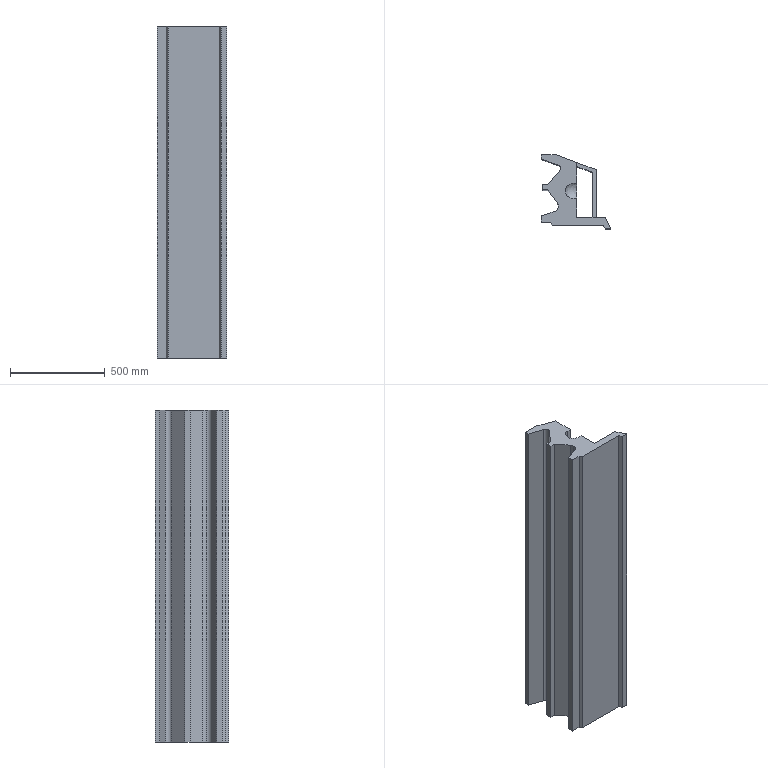Part | SolidWorks | features 3DProfileFeature 2, ICE 2, Extrusion 1, MirrorPattern 1, RevCut 1 | 1 solid | 43 faces | box 368.945 x 388.507 x 1750 mm | volume 104894918 mm3 | plane 34 | cylinder 5 | spline 2 | sphere 2 | commonest cylinder face diameters 80 x3 63.152 x2
STEP:
#1=CARTESIAN_POINT('',(-20.,75.504,-1650.));
#2=VERTEX_POINT('',#1);
#3=CARTESIAN_POINT('',(-60.,35.504,-1650.));
#4=VERTEX_POINT('',#3);
#5=CARTESIAN_POINT('',(-20.,35.504,-1650.));
#6=DIRECTION('',(0.,0.,1.));
#7=DIRECTION('',(-1.,0.,0.));
#8=AXIS2_PLACEMENT_3D('',#5,#6,#7);
#9=CIRCLE('',#8,40.);
#10=EDGE_CURVE('',#2,#4,#9,.T.);
#11=ORIENTED_EDGE('',*,*,#10,.T.);
#12=CARTESIAN_POINT('',(-60.,35.504,-1750.));
#13=VERTEX_POINT('',#12);
#14=CARTESIAN_POINT('',(-60.,35.504,-1650.));
#15=DIRECTION('',(0.,0.,-1.));
#16=VECTOR('',#15,1000.);
#17=LINE('',#14,#16);
#18=EDGE_CURVE('',#4,#13,#17,.T.);
#19=ORIENTED_EDGE('',*,*,#18,.T.);
#20=CARTESIAN_POINT('',(-20.,75.504,-1750.));
#21=VERTEX_POINT('',#20);
#22=CARTESIAN_POINT('',(-20.,35.504,-1750.));
#23=DIRECTION('',(0.,0.,1.));
#24=DIRECTION('',(-1.,0.,0.));
#25=AXIS2_PLACEMENT_3D('',#22,#23,#24);
#26=CIRCLE('',#25,40.);
#27=EDGE_CURVE('',#21,#13,#26,.T.);
#28=ORIENTED_EDGE('',*,*,#27,.F.);
#29=CARTESIAN_POINT('',(-20.,75.504,-1650.));
#30=DIRECTION('',(0.,0.,-1.));
#31=VECTOR('',#30,1000.);
#32=LINE('',#29,#31);
#33=EDGE_CURVE('',#2,#21,#32,.T.);
#34=ORIENTED_EDGE('',*,*,#33,.F.);
#35=EDGE_LOOP('',(#11,#19,#28,#34));
#36=FACE_OUTER_BOUND('',#35,.T.);
#37=CARTESIAN_POINT('',(-20.,35.504,-1650.));
#38=DIRECTION('',(0.,0.,-1.));
#39=DIRECTION('',(-1.,0.,0.));
#40=AXIS2_PLACEMENT_3D('',#37,#38,#39);
#41=CYLINDRICAL_SURFACE('',#40,40.);
#42=ADVANCED_FACE('',(#36),#41,.F.);
#43=CARTESIAN_POINT('',(-95.432,-44.492,-1750.));
#44=VERTEX_POINT('',#43);
#45=CARTESIAN_POINT('',(-102.008,-25.204,-1750.));
#46=VERTEX_POINT('',#45);
#47=CARTESIAN_POINT('',(-127.008,-44.492,-1750.));
#48=DIRECTION('',(0.,0.,1.));
#49=DIRECTION('',(1.,0.,0.));
#50=AXIS2_PLACEMENT_3D('',#47,#48,#49);
#51=CIRCLE('',#50,31.576);
#52=EDGE_CURVE('',#44,#46,#51,.T.);
#53=ORIENTED_EDGE('',*,*,#52,.F.);
#54=CARTESIAN_POINT('',(-95.432,-44.492,0.));
#55=VERTEX_POINT('',#54);
#56=CARTESIAN_POINT('',(-95.432,-44.492,-1750.));
#57=DIRECTION('',(0.,0.,1.));
#58=VECTOR('',#57,1000.);
#59=LINE('',#56,#58);
#60=EDGE_CURVE('',#44,#55,#59,.T.);
#61=ORIENTED_EDGE('',*,*,#60,.T.);
#62=CARTESIAN_POINT('',(-102.008,-25.204,0.));
#63=VERTEX_POINT('',#62);
#64=CARTESIAN_POINT('',(-127.008,-44.492,0.));
#65=DIRECTION('',(0.,0.,1.));
#66=DIRECTION('',(1.,0.,0.));
#67=AXIS2_PLACEMENT_3D('',#64,#65,#66);
#68=CIRCLE('',#67,31.576);
#69=EDGE_CURVE('',#55,#63,#68,.T.);
#70=ORIENTED_EDGE('',*,*,#69,.T.);
#71=CARTESIAN_POINT('',(-102.008,-25.204,-1750.));
#72=DIRECTION('',(0.,0.,1.));
#73=VECTOR('',#72,1000.);
#74=LINE('',#71,#73);
#75=EDGE_CURVE('',#46,#63,#74,.T.);
#76=ORIENTED_EDGE('',*,*,#75,.F.);
#77=EDGE_LOOP('',(#53,#61,#70,#76));
#78=FACE_OUTER_BOUND('',#77,.T.);
#79=CARTESIAN_POINT('',(-127.008,-44.492,-1750.));
#80=DIRECTION('',(0.,0.,1.));
#81=DIRECTION('',(1.,0.,0.));
#82=AXIS2_PLACEMENT_3D('',#79,#80,#81);
#83=CYLINDRICAL_SURFACE('',#82,31.576);
#84=ADVANCED_FACE('',(#78),#83,.F.);
#85=CARTESIAN_POINT('',(0.,185.504,-1590.));
#86=VERTEX_POINT('',#85);
#87=CARTESIAN_POINT('',(0.,164.598,-1590.));
#88=VERTEX_POINT('',#87);
#89=CARTESIAN_POINT('',(0.,164.598,-1590.));
#90=DIRECTION('',(0.,-1.,0.));
#91=VECTOR('',#90,1000.);
#92=LINE('',#89,#91);
#93=EDGE_CURVE('',#86,#88,#92,.T.);
#94=ORIENTED_EDGE('',*,*,#93,.T.);
#95=CARTESIAN_POINT('',(0.,164.598,-160.));
#96=VERTEX_POINT('',#95);
#97=CARTESIAN_POINT('',(0.,164.598,-1590.));
#98=DIRECTION('',(0.,0.,1.));
#99=VECTOR('',#98,1000.);
#100=LINE('',#97,#99);
#101=EDGE_CURVE('',#88,#96,#100,.T.);
#102=ORIENTED_EDGE('',*,*,#101,.T.);
#103=CARTESIAN_POINT('',(0.,185.504,-160.));
#104=VERTEX_POINT('',#103);
#105=CARTESIAN_POINT('',(0.,164.598,-160.));
#106=DIRECTION('',(0.,-1.,0.));
#107=VECTOR('',#106,1000.);
#108=LINE('',#105,#107);
#109=EDGE_CURVE('',#104,#96,#108,.T.);
#110=ORIENTED_EDGE('',*,*,#109,.F.);
#111=CARTESIAN_POINT('',(0.,185.504,0.));
#112=VERTEX_POINT('',#111);
#113=CARTESIAN_POINT('',(0.,185.504,-1750.));
#114=DIRECTION('',(0.,0.,1.));
#115=VECTOR('',#114,1000.);
#116=LINE('',#113,#115);
#117=EDGE_CURVE('',#104,#112,#116,.T.);
#118=ORIENTED_EDGE('',*,*,#117,.T.);
#119=CARTESIAN_POINT('',(0.,75.504,0.));
#120=VERTEX_POINT('',#119);
#121=CARTESIAN_POINT('',(0.,0.,0.));
#122=DIRECTION('',(0.,-1.,0.));
#123=VECTOR('',#122,1000.);
#124=LINE('',#121,#123);
#125=EDGE_CURVE('',#112,#120,#124,.T.);
#126=ORIENTED_EDGE('',*,*,#125,.T.);
#127=CARTESIAN_POINT('',(0.,75.504,-100.));
#128=VERTEX_POINT('',#127);
#129=CARTESIAN_POINT('',(0.,75.504,-100.));
#130=DIRECTION('',(0.,0.,1.));
#131=VECTOR('',#130,1000.);
#132=LINE('',#129,#131);
#133=EDGE_CURVE('',#128,#120,#132,.T.);
#134=ORIENTED_EDGE('',*,*,#133,.F.);
#135=CARTESIAN_POINT('',(0.,95.504,-100.));
#136=VERTEX_POINT('',#135);
#137=CARTESIAN_POINT('',(0.,95.504,-100.));
#138=DIRECTION('',(0.,-1.,0.));
#139=VECTOR('',#138,1000.);
#140=LINE('',#137,#139);
#141=EDGE_CURVE('',#136,#128,#140,.T.);
#142=ORIENTED_EDGE('',*,*,#141,.F.);
#143=CARTESIAN_POINT('',(0.,-24.496,-100.));
#144=VERTEX_POINT('',#143);
#145=CARTESIAN_POINT('',(0.,35.504,-100.));
#146=DIRECTION('',(1.,0.,0.));
#147=DIRECTION('',(0.,-1.,0.));
#148=AXIS2_PLACEMENT_3D('',#145,#146,#147);
#149=CIRCLE('',#148,60.);
#150=EDGE_CURVE('',#144,#136,#149,.T.);
#151=ORIENTED_EDGE('',*,*,#150,.F.);
#152=CARTESIAN_POINT('',(0.,-4.496,-100.));
#153=VERTEX_POINT('',#152);
#154=CARTESIAN_POINT('',(0.,95.504,-100.));
#155=DIRECTION('',(0.,-1.,0.));
#156=VECTOR('',#155,1000.);
#157=LINE('',#154,#156);
#158=EDGE_CURVE('',#153,#144,#157,.T.);
#159=ORIENTED_EDGE('',*,*,#158,.F.);
#160=CARTESIAN_POINT('',(0.,-4.496,0.));
#161=VERTEX_POINT('',#160);
#162=CARTESIAN_POINT('',(0.,-4.496,-100.));
#163=DIRECTION('',(0.,0.,1.));
#164=VECTOR('',#163,1000.);
#165=LINE('',#162,#164);
#166=EDGE_CURVE('',#153,#161,#165,.T.);
#167=ORIENTED_EDGE('',*,*,#166,.T.);
#168=CARTESIAN_POINT('',(0.,-104.496,0.));
#169=VERTEX_POINT('',#168);
#170=CARTESIAN_POINT('',(0.,0.,0.));
#171=DIRECTION('',(0.,-1.,0.));
#172=VECTOR('',#171,1000.);
#173=LINE('',#170,#172);
#174=EDGE_CURVE('',#161,#169,#173,.T.);
#175=ORIENTED_EDGE('',*,*,#174,.T.);
#176=CARTESIAN_POINT('',(0.,-104.496,-1750.));
#177=VERTEX_POINT('',#176);
#178=CARTESIAN_POINT('',(0.,-104.496,-1750.));
#179=DIRECTION('',(0.,0.,1.));
#180=VECTOR('',#179,1000.);
#181=LINE('',#178,#180);
#182=EDGE_CURVE('',#177,#169,#181,.T.);
#183=ORIENTED_EDGE('',*,*,#182,.F.);
#184=CARTESIAN_POINT('',(0.,-4.496,-1750.));
#185=VERTEX_POINT('',#184);
#186=CARTESIAN_POINT('',(0.,0.,-1750.));
#187=DIRECTION('',(0.,-1.,0.));
#188=VECTOR('',#187,1000.);
#189=LINE('',#186,#188);
#190=EDGE_CURVE('',#185,#177,#189,.T.);
#191=ORIENTED_EDGE('',*,*,#190,.F.);
#192=CARTESIAN_POINT('',(0.,-4.496,-1650.));
#193=VERTEX_POINT('',#192);
#194=CARTESIAN_POINT('',(0.,-4.496,-1650.));
#195=DIRECTION('',(0.,0.,-1.));
#196=VECTOR('',#195,1000.);
#197=LINE('',#194,#196);
#198=EDGE_CURVE('',#193,#185,#197,.T.);
#199=ORIENTED_EDGE('',*,*,#198,.F.);
#200=CARTESIAN_POINT('',(0.,-24.496,-1650.));
#201=VERTEX_POINT('',#200);
#202=CARTESIAN_POINT('',(0.,95.504,-1650.));
#203=DIRECTION('',(0.,-1.,0.));
#204=VECTOR('',#203,1000.);
#205=LINE('',#202,#204);
#206=EDGE_CURVE('',#193,#201,#205,.T.);
#207=ORIENTED_EDGE('',*,*,#206,.T.);
#208=CARTESIAN_POINT('',(0.,95.504,-1650.));
#209=VERTEX_POINT('',#208);
#210=CARTESIAN_POINT('',(0.,35.504,-1650.));
#211=DIRECTION('',(-1.,0.,0.));
#212=DIRECTION('',(0.,-1.,0.));
#213=AXIS2_PLACEMENT_3D('',#210,#211,#212);
#214=CIRCLE('',#213,60.);
#215=EDGE_CURVE('',#201,#209,#214,.T.);
#216=ORIENTED_EDGE('',*,*,#215,.T.);
#217=CARTESIAN_POINT('',(0.,75.504,-1650.));
#218=VERTEX_POINT('',#217);
#219=CARTESIAN_POINT('',(0.,95.504,-1650.));
#220=DIRECTION('',(0.,-1.,0.));
#221=VECTOR('',#220,1000.);
#222=LINE('',#219,#221);
#223=EDGE_CURVE('',#209,#218,#222,.T.);
#224=ORIENTED_EDGE('',*,*,#223,.T.);
#225=CARTESIAN_POINT('',(0.,75.504,-1750.));
#226=VERTEX_POINT('',#225);
#227=CARTESIAN_POINT('',(0.,75.504,-1650.));
#228=DIRECTION('',(0.,0.,-1.));
#229=VECTOR('',#228,1000.);
#230=LINE('',#227,#229);
#231=EDGE_CURVE('',#218,#226,#230,.T.);
#232=ORIENTED_EDGE('',*,*,#231,.T.);
#233=CARTESIAN_POINT('',(0.,185.504,-1750.));
#234=VERTEX_POINT('',#233);
#235=CARTESIAN_POINT('',(0.,0.,-1750.));
#236=DIRECTION('',(0.,-1.,0.));
#237=VECTOR('',#236,1000.);
#238=LINE('',#235,#237);
#239=EDGE_CURVE('',#234,#226,#238,.T.);
#240=ORIENTED_EDGE('',*,*,#239,.F.);
#241=CARTESIAN_POINT('',(0.,185.504,-1750.));
#242=DIRECTION('',(0.,0.,1.));
#243=VECTOR('',#242,1000.);
#244=LINE('',#241,#243);
#245=EDGE_CURVE('',#234,#86,#244,.T.);
#246=ORIENTED_EDGE('',*,*,#245,.T.);
#247=EDGE_LOOP('',(#94,#102,#110,#118,#126,#134,#142,#151,#159,#167,#175,#183,#191,#199,#207,#216,#224,#232,#240,#246));
#248=FACE_OUTER_BOUND('',#247,.T.);
#249=CARTESIAN_POINT('',(0.,0.,-1750.));
#250=DIRECTION('',(-1.,0.,0.));
#251=DIRECTION('',(0.,-1.,0.));
#252=AXIS2_PLACEMENT_3D('',#249,#250,#251);
#253=PLANE('',#252);
#254=ADVANCED_FACE('',(#248),#253,.F.);
#255=CARTESIAN_POINT('',(150.772,-104.496,0.));
#256=VERTEX_POINT('',#255);
#257=CARTESIAN_POINT('',(0.,-104.496,0.));
#258=DIRECTION('',(1.,0.,0.));
#259=VECTOR('',#258,1000.);
#260=LINE('',#257,#259);
#261=EDGE_CURVE('',#169,#256,#260,.T.);
#262=ORIENTED_EDGE('',*,*,#261,.T.);
#263=CARTESIAN_POINT('',(150.772,-104.496,-1750.));
#264=VERTEX_POINT('',#263);
#265=CARTESIAN_POINT('',(150.772,-104.496,-1750.));
#266=DIRECTION('',(0.,0.,1.));
#267=VECTOR('',#266,1000.);
#268=LINE('',#265,#267);
#269=EDGE_CURVE('',#264,#256,#268,.T.);
#270=ORIENTED_EDGE('',*,*,#269,.F.);
#271=CARTESIAN_POINT('',(0.,-104.496,-1750.));
#272=DIRECTION('',(1.,0.,0.));
#273=VECTOR('',#272,1000.);
#274=LINE('',#271,#273);
#275=EDGE_CURVE('',#177,#264,#274,.T.);
#276=ORIENTED_EDGE('',*,*,#275,.F.);
#277=ORIENTED_EDGE('',*,*,#182,.T.);
#278=EDGE_LOOP('',(#262,#270,#276,#277));
#279=FACE_OUTER_BOUND('',#278,.T.);
#280=CARTESIAN_POINT('',(83.175,-104.496,-1590.));
#281=VERTEX_POINT('',#280);
#282=CARTESIAN_POINT('',(103.143,-104.496,-1590.));
#283=VERTEX_POINT('',#282);
#284=CARTESIAN_POINT('',(103.143,-104.496,-1590.));
#285=DIRECTION('',(1.,0.,0.));
#286=VECTOR('',#285,1000.);
#287=LINE('',#284,#286);
#288=EDGE_CURVE('',#281,#283,#287,.T.);
#289=ORIENTED_EDGE('',*,*,#288,.T.);
#290=CARTESIAN_POINT('',(103.143,-104.496,-160.));
#291=VERTEX_POINT('',#290);
#292=CARTESIAN_POINT('',(103.143,-104.496,-1590.));
#293=DIRECTION('',(0.,0.,1.));
#294=VECTOR('',#293,1000.);
#295=LINE('',#292,#294);
#296=EDGE_CURVE('',#283,#291,#295,.T.);
#297=ORIENTED_EDGE('',*,*,#296,.T.);
#298=CARTESIAN_POINT('',(83.175,-104.496,-160.));
#299=VERTEX_POINT('',#298);
#300=CARTESIAN_POINT('',(103.143,-104.496,-160.));
#301=DIRECTION('',(1.,0.,0.));
#302=VECTOR('',#301,1000.);
#303=LINE('',#300,#302);
#304=EDGE_CURVE('',#299,#291,#303,.T.);
#305=ORIENTED_EDGE('',*,*,#304,.F.);
#306=CARTESIAN_POINT('',(83.175,-104.496,-1590.));
#307=DIRECTION('',(0.,0.,1.));
#308=VECTOR('',#307,1000.);
#309=LINE('',#306,#308);
#310=EDGE_CURVE('',#281,#299,#309,.T.);
#311=ORIENTED_EDGE('',*,*,#310,.F.);
#312=EDGE_LOOP('',(#289,#297,#305,#311));
#313=FACE_BOUND('',#312,.T.);
#314=CARTESIAN_POINT('',(0.,-104.496,-1750.));
#315=DIRECTION('',(0.,-1.,0.));
#316=DIRECTION('',(0.,0.,-1.));
#317=AXIS2_PLACEMENT_3D('',#314,#315,#316);
#318=PLANE('',#317);
#319=ADVANCED_FACE('',(#279,#313),#318,.F.);
#320=CARTESIAN_POINT('',(-99.707,172.982,0.));
#321=VERTEX_POINT('',#320);
#322=CARTESIAN_POINT('',(-185.497,202.508,0.));
#323=VERTEX_POINT('',#322);
#324=CARTESIAN_POINT('',(42.67,123.982,0.));
#325=DIRECTION('',(-0.9456,0.3254,0.));
#326=VECTOR('',#325,1000.);
#327=LINE('',#324,#326);
#328=EDGE_CURVE('',#321,#323,#327,.T.);
#329=ORIENTED_EDGE('',*,*,#328,.T.);
#330=CARTESIAN_POINT('',(-185.497,202.508,-1750.));
#331=VERTEX_POINT('',#330);
#332=CARTESIAN_POINT('',(-185.497,202.508,-1750.));
#333=DIRECTION('',(0.,0.,1.));
#334=VECTOR('',#333,1000.);
#335=LINE('',#332,#334);
#336=EDGE_CURVE('',#331,#323,#335,.T.);
#337=ORIENTED_EDGE('',*,*,#336,.F.);
#338=CARTESIAN_POINT('',(-99.707,172.982,-1750.));
#339=VERTEX_POINT('',#338);
#340=CARTESIAN_POINT('',(42.67,123.982,-1750.));
#341=DIRECTION('',(-0.9456,0.3254,0.));
#342=VECTOR('',#341,1000.);
#343=LINE('',#340,#342);
#344=EDGE_CURVE('',#339,#331,#343,.T.);
#345=ORIENTED_EDGE('',*,*,#344,.F.);
#346=CARTESIAN_POINT('',(-99.707,172.982,-1750.));
#347=DIRECTION('',(0.,0.,1.));
#348=VECTOR('',#347,1000.);
#349=LINE('',#346,#348);
#350=EDGE_CURVE('',#339,#321,#349,.T.);
#351=ORIENTED_EDGE('',*,*,#350,.T.);
#352=EDGE_LOOP('',(#329,#337,#345,#351));
#353=FACE_OUTER_BOUND('',#352,.T.);
#354=CARTESIAN_POINT('',(42.67,123.982,-1750.));
#355=DIRECTION('',(0.3254,0.9456,0.));
#356=DIRECTION('',(-0.9456,0.3254,0.));
#357=AXIS2_PLACEMENT_3D('',#354,#355,#356);
#358=PLANE('',#357);
#359=ADVANCED_FACE('',(#353),#358,.F.);
#360=CARTESIAN_POINT('',(-185.497,225.508,0.));
#361=VERTEX_POINT('',#360);
#362=CARTESIAN_POINT('',(-185.497,0.,0.));
#363=DIRECTION('',(0.,1.,0.));
#364=VECTOR('',#363,1000.);
#365=LINE('',#362,#364);
#366=EDGE_CURVE('',#323,#361,#365,.T.);
#367=ORIENTED_EDGE('',*,*,#366,.T.);
#368=CARTESIAN_POINT('',(-185.497,225.508,-1750.));
#369=VERTEX_POINT('',#368);
#370=CARTESIAN_POINT('',(-185.497,225.508,-1750.));
#371=DIRECTION('',(0.,0.,1.));
#372=VECTOR('',#371,1000.);
#373=LINE('',#370,#372);
#374=EDGE_CURVE('',#369,#361,#373,.T.);
#375=ORIENTED_EDGE('',*,*,#374,.F.);
#376=CARTESIAN_POINT('',(-185.497,0.,-1750.));
#377=DIRECTION('',(0.,1.,0.));
#378=VECTOR('',#377,1000.);
#379=LINE('',#376,#378);
#380=EDGE_CURVE('',#331,#369,#379,.T.);
#381=ORIENTED_EDGE('',*,*,#380,.F.);
#382=ORIENTED_EDGE('',*,*,#336,.T.);
#383=EDGE_LOOP('',(#367,#375,#381,#382));
#384=FACE_OUTER_BOUND('',#383,.T.);
#385=CARTESIAN_POINT('',(-185.497,0.,-1750.));
#386=DIRECTION('',(1.,0.,0.));
#387=DIRECTION('',(0.,0.,-1.));
#388=AXIS2_PLACEMENT_3D('',#385,#386,#387);
#389=PLANE('',#388);
#390=ADVANCED_FACE('',(#384),#389,.F.);
#391=CARTESIAN_POINT('',(-107.777,225.508,0.));
#392=VERTEX_POINT('',#391);
#393=CARTESIAN_POINT('',(0.,225.508,0.));
#394=DIRECTION('',(1.,0.,0.));
#395=VECTOR('',#394,1000.);
#396=LINE('',#393,#395);
#397=EDGE_CURVE('',#361,#392,#396,.T.);
#398=ORIENTED_EDGE('',*,*,#397,.T.);
#399=CARTESIAN_POINT('',(-107.777,225.508,-1750.));
#400=VERTEX_POINT('',#399);
#401=CARTESIAN_POINT('',(-107.777,225.508,-1750.));
#402=DIRECTION('',(0.,0.,1.));
#403=VECTOR('',#402,1000.);
#404=LINE('',#401,#403);
#405=EDGE_CURVE('',#400,#392,#404,.T.);
#406=ORIENTED_EDGE('',*,*,#405,.F.);
#407=CARTESIAN_POINT('',(0.,225.508,-1750.));
#408=DIRECTION('',(1.,0.,0.));
#409=VECTOR('',#408,1000.);
#410=LINE('',#407,#409);
#411=EDGE_CURVE('',#369,#400,#410,.T.);
#412=ORIENTED_EDGE('',*,*,#411,.F.);
#413=ORIENTED_EDGE('',*,*,#374,.T.);
#414=EDGE_LOOP('',(#398,#406,#412,#413));
#415=FACE_OUTER_BOUND('',#414,.T.);
#416=CARTESIAN_POINT('',(0.,225.508,-1750.));
#417=DIRECTION('',(0.,-1.,0.));
#418=DIRECTION('',(0.,0.,-1.));
#419=AXIS2_PLACEMENT_3D('',#416,#417,#418);
#420=PLANE('',#419);
#421=ADVANCED_FACE('',(#415),#420,.F.);
#422=CARTESIAN_POINT('',(60.517,163.042,0.));
#423=DIRECTION('',(0.9375,-0.348,0.));
#424=VECTOR('',#423,1000.);
#425=LINE('',#422,#424);
#426=EDGE_CURVE('',#392,#112,#425,.T.);
#427=ORIENTED_EDGE('',*,*,#426,.T.);
#428=ORIENTED_EDGE('',*,*,#117,.F.);
#429=CARTESIAN_POINT('',(103.143,147.22,-160.));
#430=VERTEX_POINT('',#429);
#431=CARTESIAN_POINT('',(0.,185.504,-160.));
#432=DIRECTION('',(-0.9375,0.348,0.));
#433=VECTOR('',#432,1000.);
#434=LINE('',#431,#433);
#435=EDGE_CURVE('',#430,#104,#434,.T.);
#436=ORIENTED_EDGE('',*,*,#435,.F.);
#437=CARTESIAN_POINT('',(103.143,147.22,-1590.));
#438=VERTEX_POINT('',#437);
#439=CARTESIAN_POINT('',(103.143,147.22,-1590.));
#440=DIRECTION('',(0.,0.,1.));
#441=VECTOR('',#440,1000.);
#442=LINE('',#439,#441);
#443=EDGE_CURVE('',#438,#430,#442,.T.);
#444=ORIENTED_EDGE('',*,*,#443,.F.);
#445=CARTESIAN_POINT('',(63.207,162.043,-1590.));
#446=DIRECTION('',(-0.9375,0.348,0.));
#447=VECTOR('',#446,1000.);
#448=LINE('',#445,#447);
#449=EDGE_CURVE('',#438,#86,#448,.T.);
#450=ORIENTED_EDGE('',*,*,#449,.T.);
#451=ORIENTED_EDGE('',*,*,#245,.F.);
#452=CARTESIAN_POINT('',(60.517,163.042,-1750.));
#453=DIRECTION('',(0.9375,-0.348,0.));
#454=VECTOR('',#453,1000.);
#455=LINE('',#452,#454);
#456=EDGE_CURVE('',#400,#234,#455,.T.);
#457=ORIENTED_EDGE('',*,*,#456,.F.);
#458=ORIENTED_EDGE('',*,*,#405,.T.);
#459=EDGE_LOOP('',(#427,#428,#436,#444,#450,#451,#457,#458));
#460=FACE_OUTER_BOUND('',#459,.T.);
#461=CARTESIAN_POINT('',(60.517,163.042,-1750.));
#462=DIRECTION('',(-0.348,-0.9375,0.));
#463=DIRECTION('',(0.9375,-0.348,0.));
#464=AXIS2_PLACEMENT_3D('',#461,#462,#463);
#465=PLANE('',#464);
#466=ADVANCED_FACE('',(#460),#465,.F.);
#467=CARTESIAN_POINT('',(180.948,-163.,0.));
#468=VERTEX_POINT('',#467);
#469=CARTESIAN_POINT('',(76.518,39.467,0.));
#470=DIRECTION('',(-0.4584,0.8887,0.));
#471=VECTOR('',#470,1000.);
#472=LINE('',#469,#471);
#473=EDGE_CURVE('',#468,#256,#472,.T.);
#474=ORIENTED_EDGE('',*,*,#473,.F.);
#475=CARTESIAN_POINT('',(180.948,-163.,-1750.));
#476=VERTEX_POINT('',#475);
#477=CARTESIAN_POINT('',(180.948,-163.,-1750.));
#478=DIRECTION('',(0.,0.,1.));
#479=VECTOR('',#478,1000.);
#480=LINE('',#477,#479);
#481=EDGE_CURVE('',#476,#468,#480,.T.);
#482=ORIENTED_EDGE('',*,*,#481,.F.);
#483=CARTESIAN_POINT('',(76.518,39.467,-1750.));
#484=DIRECTION('',(-0.4584,0.8887,0.));
#485=VECTOR('',#484,1000.);
#486=LINE('',#483,#485);
#487=EDGE_CURVE('',#476,#264,#486,.T.);
#488=ORIENTED_EDGE('',*,*,#487,.T.);
#489=ORIENTED_EDGE('',*,*,#269,.T.);
#490=EDGE_LOOP('',(#474,#482,#488,#489));
#491=FACE_OUTER_BOUND('',#490,.T.);
#492=CARTESIAN_POINT('',(76.518,39.467,-1750.));
#493=DIRECTION('',(0.8887,0.4584,0.));
#494=DIRECTION('',(-0.4584,0.8887,0.));
#495=AXIS2_PLACEMENT_3D('',#492,#493,#494);
#496=PLANE('',#495);
#497=ADVANCED_FACE('',(#491),#496,.T.);
#498=CARTESIAN_POINT('',(150.772,-163.,0.));
#499=VERTEX_POINT('',#498);
#500=CARTESIAN_POINT('',(0.,-163.,0.));
#501=DIRECTION('',(1.,0.,0.));
#502=VECTOR('',#501,1000.);
#503=LINE('',#500,#502);
#504=EDGE_CURVE('',#499,#468,#503,.T.);
#505=ORIENTED_EDGE('',*,*,#504,.F.);
#506=CARTESIAN_POINT('',(150.772,-163.,-1750.));
#507=VERTEX_POINT('',#506);
#508=CARTESIAN_POINT('',(150.772,-163.,-1750.));
#509=DIRECTION('',(0.,0.,1.));
#510=VECTOR('',#509,1000.);
#511=LINE('',#508,#510);
#512=EDGE_CURVE('',#507,#499,#511,.T.);
#513=ORIENTED_EDGE('',*,*,#512,.F.);
#514=CARTESIAN_POINT('',(0.,-163.,-1750.));
#515=DIRECTION('',(1.,0.,0.));
#516=VECTOR('',#515,1000.);
#517=LINE('',#514,#516);
#518=EDGE_CURVE('',#507,#476,#517,.T.);
#519=ORIENTED_EDGE('',*,*,#518,.T.);
#520=ORIENTED_EDGE('',*,*,#481,.T.);
#521=EDGE_LOOP('',(#505,#513,#519,#520));
#522=FACE_OUTER_BOUND('',#521,.T.);
#523=CARTESIAN_POINT('',(0.,-163.,-1750.));
#524=DIRECTION('',(0.,-1.,0.));
#525=DIRECTION('',(0.,0.,-1.));
#526=AXIS2_PLACEMENT_3D('',#523,#524,#525);
#527=PLANE('',#526);
#528=ADVANCED_FACE('',(#522),#527,.T.);
#529=CARTESIAN_POINT('',(140.,-144.496,0.));
#530=VERTEX_POINT('',#529);
#531=CARTESIAN_POINT('',(41.734,24.296,0.));
#532=DIRECTION('',(0.5031,-0.8642,0.));
#533=VECTOR('',#532,1000.);
#534=LINE('',#531,#533);
#535=EDGE_CURVE('',#530,#499,#534,.T.);
#536=ORIENTED_EDGE('',*,*,#535,.F.);
#537=CARTESIAN_POINT('',(140.,-144.496,-1750.));
#538=VERTEX_POINT('',#537);
#539=CARTESIAN_POINT('',(140.,-144.496,-1750.));
#540=DIRECTION('',(0.,0.,1.));
#541=VECTOR('',#540,1000.);
#542=LINE('',#539,#541);
#543=EDGE_CURVE('',#538,#530,#542,.T.);
#544=ORIENTED_EDGE('',*,*,#543,.F.);
#545=CARTESIAN_POINT('',(41.734,24.296,-1750.));
#546=DIRECTION('',(0.5031,-0.8642,0.));
#547=VECTOR('',#546,1000.);
#548=LINE('',#545,#547);
#549=EDGE_CURVE('',#538,#507,#548,.T.);
#550=ORIENTED_EDGE('',*,*,#549,.T.);
#551=ORIENTED_EDGE('',*,*,#512,.T.);
#552=EDGE_LOOP('',(#536,#544,#550,#551));
#553=FACE_OUTER_BOUND('',#552,.T.);
#554=CARTESIAN_POINT('',(41.734,24.296,-1750.));
#555=DIRECTION('',(-0.8642,-0.5031,0.));
#556=DIRECTION('',(0.5031,-0.8642,0.));
#557=AXIS2_PLACEMENT_3D('',#554,#555,#556);
#558=PLANE('',#557);
#559=ADVANCED_FACE('',(#553),#558,.T.);
#560=CARTESIAN_POINT('',(-130.,-144.496,0.));
#561=VERTEX_POINT('',#560);
#562=CARTESIAN_POINT('',(0.,-144.496,0.));
#563=DIRECTION('',(-1.,0.,0.));
#564=VECTOR('',#563,1000.);
#565=LINE('',#562,#564);
#566=EDGE_CURVE('',#530,#561,#565,.T.);
#567=ORIENTED_EDGE('',*,*,#566,.T.);
#568=CARTESIAN_POINT('',(-130.,-144.496,-1750.));
#569=VERTEX_POINT('',#568);
#570=CARTESIAN_POINT('',(-130.,-144.496,-1750.));
#571=DIRECTION('',(0.,0.,1.));
#572=VECTOR('',#571,1000.);
#573=LINE('',#570,#572);
#574=EDGE_CURVE('',#569,#561,#573,.T.);
#575=ORIENTED_EDGE('',*,*,#574,.F.);
#576=CARTESIAN_POINT('',(0.,-144.496,-1750.));
#577=DIRECTION('',(-1.,0.,0.));
#578=VECTOR('',#577,1000.);
#579=LINE('',#576,#578);
#580=EDGE_CURVE('',#538,#569,#579,.T.);
#581=ORIENTED_EDGE('',*,*,#580,.F.);
#582=ORIENTED_EDGE('',*,*,#543,.T.);
#583=EDGE_LOOP('',(#567,#575,#581,#582));
#584=FACE_OUTER_BOUND('',#583,.T.);
#585=CARTESIAN_POINT('',(0.,-144.496,-1750.));
#586=DIRECTION('',(0.,1.,0.));
#587=DIRECTION('',(-1.,0.,0.));
#588=AXIS2_PLACEMENT_3D('',#585,#586,#587);
#589=PLANE('',#588);
#590=ADVANCED_FACE('',(#584),#589,.F.);
#591=CARTESIAN_POINT('',(-140.3,-129.496,0.));
#592=VERTEX_POINT('',#591);
#593=CARTESIAN_POINT('',(-155.774,-106.96,0.));
#594=DIRECTION('',(-0.566,0.8244,0.));
#595=VECTOR('',#594,1000.);
#596=LINE('',#593,#595);
#597=EDGE_CURVE('',#561,#592,#596,.T.);
#598=ORIENTED_EDGE('',*,*,#597,.T.);
#599=CARTESIAN_POINT('',(-140.3,-129.496,-1750.));
#600=VERTEX_POINT('',#599);
#601=CARTESIAN_POINT('',(-140.3,-129.496,-1750.));
#602=DIRECTION('',(0.,0.,1.));
#603=VECTOR('',#602,1000.);
#604=LINE('',#601,#603);
#605=EDGE_CURVE('',#600,#592,#604,.T.);
#606=ORIENTED_EDGE('',*,*,#605,.F.);
#607=CARTESIAN_POINT('',(-155.774,-106.96,-1750.));
#608=DIRECTION('',(-0.566,0.8244,0.));
#609=VECTOR('',#608,1000.);
#610=LINE('',#607,#609);
#611=EDGE_CURVE('',#569,#600,#610,.T.);
#612=ORIENTED_EDGE('',*,*,#611,.F.);
#613=ORIENTED_EDGE('',*,*,#574,.T.);
#614=EDGE_LOOP('',(#598,#606,#612,#613));
#615=FACE_OUTER_BOUND('',#614,.T.);
#616=CARTESIAN_POINT('',(-155.774,-106.96,-1750.));
#617=DIRECTION('',(0.8244,0.566,0.));
#618=DIRECTION('',(-0.566,0.8244,0.));
#619=AXIS2_PLACEMENT_3D('',#616,#617,#618);
#620=PLANE('',#619);
#621=ADVANCED_FACE('',(#615),#620,.F.);
#622=CARTESIAN_POINT('',(-187.997,-129.496,0.));
#623=VERTEX_POINT('',#622);
#624=CARTESIAN_POINT('',(0.,-129.496,0.));
#625=DIRECTION('',(-1.,0.,0.));
#626=VECTOR('',#625,1000.);
#627=LINE('',#624,#626);
#628=EDGE_CURVE('',#592,#623,#627,.T.);
#629=ORIENTED_EDGE('',*,*,#628,.T.);
#630=CARTESIAN_POINT('',(-187.997,-129.496,-1750.));
#631=VERTEX_POINT('',#630);
#632=CARTESIAN_POINT('',(-187.997,-129.496,-1750.));
#633=DIRECTION('',(0.,0.,1.));
#634=VECTOR('',#633,1000.);
#635=LINE('',#632,#634);
#636=EDGE_CURVE('',#631,#623,#635,.T.);
#637=ORIENTED_EDGE('',*,*,#636,.F.);
#638=CARTESIAN_POINT('',(0.,-129.496,-1750.));
#639=DIRECTION('',(-1.,0.,0.));
#640=VECTOR('',#639,1000.);
#641=LINE('',#638,#640);
#642=EDGE_CURVE('',#600,#631,#641,.T.);
#643=ORIENTED_EDGE('',*,*,#642,.F.);
#644=ORIENTED_EDGE('',*,*,#605,.T.);
#645=EDGE_LOOP('',(#629,#637,#643,#644));
#646=FACE_OUTER_BOUND('',#645,.T.);
#647=CARTESIAN_POINT('',(0.,-129.496,-1750.));
#648=DIRECTION('',(0.,1.,0.));
#649=DIRECTION('',(0.,0.,1.));
#650=AXIS2_PLACEMENT_3D('',#647,#648,#649);
#651=PLANE('',#650);
#652=ADVANCED_FACE('',(#646),#651,.F.);
#653=CARTESIAN_POINT('',(-187.997,-99.496,0.));
#654=VERTEX_POINT('',#653);
#655=CARTESIAN_POINT('',(-187.997,0.,0.));
#656=DIRECTION('',(0.,1.,0.));
#657=VECTOR('',#656,1000.);
#658=LINE('',#655,#657);
#659=EDGE_CURVE('',#623,#654,#658,.T.);
#660=ORIENTED_EDGE('',*,*,#659,.T.);
#661=CARTESIAN_POINT('',(-187.997,-99.496,-1750.));
#662=VERTEX_POINT('',#661);
#663=CARTESIAN_POINT('',(-187.997,-99.496,-1750.));
#664=DIRECTION('',(0.,0.,1.));
#665=VECTOR('',#664,1000.);
#666=LINE('',#663,#665);
#667=EDGE_CURVE('',#662,#654,#666,.T.);
#668=ORIENTED_EDGE('',*,*,#667,.F.);
#669=CARTESIAN_POINT('',(-187.997,0.,-1750.));
#670=DIRECTION('',(0.,1.,0.));
#671=VECTOR('',#670,1000.);
#672=LINE('',#669,#671);
#673=EDGE_CURVE('',#631,#662,#672,.T.);
#674=ORIENTED_EDGE('',*,*,#673,.F.);
#675=ORIENTED_EDGE('',*,*,#636,.T.);
#676=EDGE_LOOP('',(#660,#668,#674,#675));
#677=FACE_OUTER_BOUND('',#676,.T.);
#678=CARTESIAN_POINT('',(-187.997,0.,-1750.));
#679=DIRECTION('',(1.,0.,0.));
#680=DIRECTION('',(0.,0.,-1.));
#681=AXIS2_PLACEMENT_3D('',#678,#679,#680);
#682=PLANE('',#681);
#683=ADVANCED_FACE('',(#677),#682,.F.);
#684=CARTESIAN_POINT('',(-185.497,-96.731,0.));
#685=VERTEX_POINT('',#684);
#686=CARTESIAN_POINT('',(-187.997,-99.496,0.));
#687=CARTESIAN_POINT('',(-187.264,-97.684,0.));
#688=CARTESIAN_POINT('',(-185.497,-96.731,0.));
#689=B_SPLINE_CURVE_WITH_KNOTS('',2,(#686,#687,#688),.UNSPECIFIED.,.F.,.F.,(3,3),(0.,1.),.UNSPECIFIED.);
#690=EDGE_CURVE('',#654,#685,#689,.T.);
#691=ORIENTED_EDGE('',*,*,#690,.T.);
#692=CARTESIAN_POINT('',(-185.497,-96.731,-1750.));
#693=VERTEX_POINT('',#692);
#694=CARTESIAN_POINT('',(-185.497,-96.731,-1750.));
#695=DIRECTION('',(0.,0.,1.));
#696=VECTOR('',#695,1000.);
#697=LINE('',#694,#696);
#698=EDGE_CURVE('',#693,#685,#697,.T.);
#699=ORIENTED_EDGE('',*,*,#698,.F.);
#700=CARTESIAN_POINT('',(-187.997,-99.496,-1750.));
#701=CARTESIAN_POINT('',(-187.264,-97.684,-1750.));
#702=CARTESIAN_POINT('',(-185.497,-96.731,-1750.));
#703=B_SPLINE_CURVE_WITH_KNOTS('',2,(#700,#701,#702),.UNSPECIFIED.,.F.,.F.,(3,3),(0.,1.),.UNSPECIFIED.);
#704=EDGE_CURVE('',#662,#693,#703,.T.);
#705=ORIENTED_EDGE('',*,*,#704,.F.);
#706=ORIENTED_EDGE('',*,*,#667,.T.);
#707=EDGE_LOOP('',(#691,#699,#705,#706));
#708=FACE_OUTER_BOUND('',#707,.T.);
#709=CARTESIAN_POINT('',(-187.997,-99.496,-1750.));
#710=CARTESIAN_POINT('',(-187.997,-99.496,0.));
#711=CARTESIAN_POINT('',(-187.264,-97.684,-1750.));
#712=CARTESIAN_POINT('',(-187.264,-97.684,0.));
#713=CARTESIAN_POINT('',(-185.497,-96.731,-1750.));
#714=CARTESIAN_POINT('',(-185.497,-96.731,0.));
#715=B_SPLINE_SURFACE_WITH_KNOTS('',2,1,((#709,#710),(#711,#712),(#713,#714)),.UNSPECIFIED.,.F.,.F.,.F.,(3,3),(2,2),(0.,1.),(0.,1.),.UNSPECIFIED.);
#716=ADVANCED_FACE('',(#708),#715,.F.);
#717=CARTESIAN_POINT('',(-107.72,-69.492,0.));
#718=VERTEX_POINT('',#717);
#719=CARTESIAN_POINT('',(9.91,-28.296,0.));
#720=DIRECTION('',(0.9438,0.3305,0.));
#721=VECTOR('',#720,1000.);
#722=LINE('',#719,#721);
#723=EDGE_CURVE('',#685,#718,#722,.T.);
#724=ORIENTED_EDGE('',*,*,#723,.T.);
#725=CARTESIAN_POINT('',(-107.72,-69.492,-1750.));
#726=VERTEX_POINT('',#725);
#727=CARTESIAN_POINT('',(-107.72,-69.492,-1750.));
#728=DIRECTION('',(0.,0.,1.));
#729=VECTOR('',#728,1000.);
#730=LINE('',#727,#729);
#731=EDGE_CURVE('',#726,#718,#730,.T.);
#732=ORIENTED_EDGE('',*,*,#731,.F.);
#733=CARTESIAN_POINT('',(9.91,-28.296,-1750.));
#734=DIRECTION('',(0.9438,0.3305,0.));
#735=VECTOR('',#734,1000.);
#736=LINE('',#733,#735);
#737=EDGE_CURVE('',#693,#726,#736,.T.);
#738=ORIENTED_EDGE('',*,*,#737,.F.);
#739=ORIENTED_EDGE('',*,*,#698,.T.);
#740=EDGE_LOOP('',(#724,#732,#738,#739));
#741=FACE_OUTER_BOUND('',#740,.T.);
#742=CARTESIAN_POINT('',(9.91,-28.296,-1750.));
#743=DIRECTION('',(0.3305,-0.9438,0.));
#744=DIRECTION('',(0.9438,0.3305,0.));
#745=AXIS2_PLACEMENT_3D('',#742,#743,#744);
#746=PLANE('',#745);
#747=ADVANCED_FACE('',(#741),#746,.F.);
#748=ORIENTED_EDGE('',*,*,#60,.F.);
#749=CARTESIAN_POINT('',(-127.008,-44.492,-1750.));
#750=DIRECTION('',(0.,0.,1.));
#751=DIRECTION('',(1.,0.,0.));
#752=AXIS2_PLACEMENT_3D('',#749,#750,#751);
#753=CIRCLE('',#752,31.576);
#754=EDGE_CURVE('',#726,#44,#753,.T.);
#755=ORIENTED_EDGE('',*,*,#754,.F.);
#756=ORIENTED_EDGE('',*,*,#731,.T.);
#757=CARTESIAN_POINT('',(-127.008,-44.492,0.));
#758=DIRECTION('',(0.,0.,1.));
#759=DIRECTION('',(1.,0.,0.));
#760=AXIS2_PLACEMENT_3D('',#757,#758,#759);
#761=CIRCLE('',#760,31.576);
#762=EDGE_CURVE('',#718,#55,#761,.T.);
#763=ORIENTED_EDGE('',*,*,#762,.T.);
#764=EDGE_LOOP('',(#748,#755,#756,#763));
#765=FACE_OUTER_BOUND('',#764,.T.);
#766=CARTESIAN_POINT('',(-127.008,-44.492,-1750.));
#767=DIRECTION('',(0.,0.,1.));
#768=DIRECTION('',(1.,0.,0.));
#769=AXIS2_PLACEMENT_3D('',#766,#767,#768);
#770=CYLINDRICAL_SURFACE('',#769,31.576);
#771=ADVANCED_FACE('',(#765),#770,.F.);
#772=CARTESIAN_POINT('',(-152.707,40.508,0.));
#773=VERTEX_POINT('',#772);
#774=CARTESIAN_POINT('',(-76.134,-58.74,0.));
#775=DIRECTION('',(-0.6109,0.7917,0.));
#776=VECTOR('',#775,1000.);
#777=LINE('',#774,#776);
#778=EDGE_CURVE('',#63,#773,#777,.T.);
#779=ORIENTED_EDGE('',*,*,#778,.T.);
#780=CARTESIAN_POINT('',(-152.707,40.508,-1750.));
#781=VERTEX_POINT('',#780);
#782=CARTESIAN_POINT('',(-152.707,40.508,-1750.));
#783=DIRECTION('',(0.,0.,1.));
#784=VECTOR('',#783,1000.);
#785=LINE('',#782,#784);
#786=EDGE_CURVE('',#781,#773,#785,.T.);
#787=ORIENTED_EDGE('',*,*,#786,.F.);
#788=CARTESIAN_POINT('',(-76.134,-58.74,-1750.));
#789=DIRECTION('',(-0.6109,0.7917,0.));
#790=VECTOR('',#789,1000.);
#791=LINE('',#788,#790);
#792=EDGE_CURVE('',#46,#781,#791,.T.);
#793=ORIENTED_EDGE('',*,*,#792,.F.);
#794=ORIENTED_EDGE('',*,*,#75,.T.);
#795=EDGE_LOOP('',(#779,#787,#793,#794));
#796=FACE_OUTER_BOUND('',#795,.T.);
#797=CARTESIAN_POINT('',(-76.134,-58.74,-1750.));
#798=DIRECTION('',(0.7917,0.6109,0.));
#799=DIRECTION('',(-0.6109,0.7917,0.));
#800=AXIS2_PLACEMENT_3D('',#797,#798,#799);
#801=PLANE('',#800);
#802=ADVANCED_FACE('',(#796),#801,.F.);
#803=CARTESIAN_POINT('',(-179.707,40.508,0.));
#804=VERTEX_POINT('',#803);
#805=CARTESIAN_POINT('',(0.,40.508,0.));
#806=DIRECTION('',(-1.,0.,0.));
#807=VECTOR('',#806,1000.);
#808=LINE('',#805,#807);
#809=EDGE_CURVE('',#773,#804,#808,.T.);
#810=ORIENTED_EDGE('',*,*,#809,.T.);
#811=CARTESIAN_POINT('',(-179.707,40.508,-1750.));
#812=VERTEX_POINT('',#811);
#813=CARTESIAN_POINT('',(-179.707,40.508,-1750.));
#814=DIRECTION('',(0.,0.,1.));
#815=VECTOR('',#814,1000.);
#816=LINE('',#813,#815);
#817=EDGE_CURVE('',#812,#804,#816,.T.);
#818=ORIENTED_EDGE('',*,*,#817,.F.);
#819=CARTESIAN_POINT('',(0.,40.508,-1750.));
#820=DIRECTION('',(-1.,0.,0.));
#821=VECTOR('',#820,1000.);
#822=LINE('',#819,#821);
#823=EDGE_CURVE('',#781,#812,#822,.T.);
#824=ORIENTED_EDGE('',*,*,#823,.F.);
#825=ORIENTED_EDGE('',*,*,#786,.T.);
#826=EDGE_LOOP('',(#810,#818,#824,#825));
#827=FACE_OUTER_BOUND('',#826,.T.);
#828=CARTESIAN_POINT('',(0.,40.508,-1750.));
#829=DIRECTION('',(0.,1.,0.));
#830=DIRECTION('',(-1.,0.,0.));
#831=AXIS2_PLACEMENT_3D('',#828,#829,#830);
#832=PLANE('',#831);
#833=ADVANCED_FACE('',(#827),#832,.F.);
#834=CARTESIAN_POINT('',(-179.707,70.508,0.));
#835=VERTEX_POINT('',#834);
#836=CARTESIAN_POINT('',(-179.707,0.,0.));
#837=DIRECTION('',(0.,1.,0.));
#838=VECTOR('',#837,1000.);
#839=LINE('',#836,#838);
#840=EDGE_CURVE('',#804,#835,#839,.T.);
#841=ORIENTED_EDGE('',*,*,#840,.T.);
#842=CARTESIAN_POINT('',(-179.707,70.508,-1750.));
#843=VERTEX_POINT('',#842);
#844=CARTESIAN_POINT('',(-179.707,70.508,-1750.));
#845=DIRECTION('',(0.,0.,1.));
#846=VECTOR('',#845,1000.);
#847=LINE('',#844,#846);
#848=EDGE_CURVE('',#843,#835,#847,.T.);
#849=ORIENTED_EDGE('',*,*,#848,.F.);
#850=CARTESIAN_POINT('',(-179.707,0.,-1750.));
#851=DIRECTION('',(0.,1.,0.));
#852=VECTOR('',#851,1000.);
#853=LINE('',#850,#852);
#854=EDGE_CURVE('',#812,#843,#853,.T.);
#855=ORIENTED_EDGE('',*,*,#854,.F.);
#856=ORIENTED_EDGE('',*,*,#817,.T.);
#857=EDGE_LOOP('',(#841,#849,#855,#856));
#858=FACE_OUTER_BOUND('',#857,.T.);
#859=CARTESIAN_POINT('',(-179.707,0.,-1750.));
#860=DIRECTION('',(1.,0.,0.));
#861=DIRECTION('',(0.,0.,-1.));
#862=AXIS2_PLACEMENT_3D('',#859,#860,#861);
#863=PLANE('',#862);
#864=ADVANCED_FACE('',(#858),#863,.F.);
#865=CARTESIAN_POINT('',(-152.707,70.508,0.));
#866=VERTEX_POINT('',#865);
#867=CARTESIAN_POINT('',(0.,70.508,0.));
#868=DIRECTION('',(1.,0.,0.));
#869=VECTOR('',#868,1000.);
#870=LINE('',#867,#869);
#871=EDGE_CURVE('',#835,#866,#870,.T.);
#872=ORIENTED_EDGE('',*,*,#871,.T.);
#873=CARTESIAN_POINT('',(-152.707,70.508,-1750.));
#874=VERTEX_POINT('',#873);
#875=CARTESIAN_POINT('',(-152.707,70.508,-1750.));
#876=DIRECTION('',(0.,0.,1.));
#877=VECTOR('',#876,1000.);
#878=LINE('',#875,#877);
#879=EDGE_CURVE('',#874,#866,#878,.T.);
#880=ORIENTED_EDGE('',*,*,#879,.F.);
#881=CARTESIAN_POINT('',(0.,70.508,-1750.));
#882=DIRECTION('',(1.,0.,0.));
#883=VECTOR('',#882,1000.);
#884=LINE('',#881,#883);
#885=EDGE_CURVE('',#843,#874,#884,.T.);
#886=ORIENTED_EDGE('',*,*,#885,.F.);
#887=ORIENTED_EDGE('',*,*,#848,.T.);
#888=EDGE_LOOP('',(#872,#880,#886,#887));
#889=FACE_OUTER_BOUND('',#888,.T.);
#890=CARTESIAN_POINT('',(0.,70.508,-1750.));
#891=DIRECTION('',(0.,-1.,0.));
#892=DIRECTION('',(0.,0.,-1.));
#893=AXIS2_PLACEMENT_3D('',#890,#891,#892);
#894=PLANE('',#893);
#895=ADVANCED_FACE('',(#889),#894,.F.);
#896=CARTESIAN_POINT('',(-92.317,140.109,0.));
#897=VERTEX_POINT('',#896);
#898=CARTESIAN_POINT('',(-122.021,105.874,0.));
#899=DIRECTION('',(-0.6554,-0.7553,0.));
#900=VECTOR('',#899,1000.);
#901=LINE('',#898,#900);
#902=EDGE_CURVE('',#897,#866,#901,.T.);
#903=ORIENTED_EDGE('',*,*,#902,.F.);
#904=CARTESIAN_POINT('',(-92.317,140.109,-1750.));
#905=VERTEX_POINT('',#904);
#906=CARTESIAN_POINT('',(-92.317,140.109,-1750.));
#907=DIRECTION('',(0.,0.,1.));
#908=VECTOR('',#907,1000.);
#909=LINE('',#906,#908);
#910=EDGE_CURVE('',#905,#897,#909,.T.);
#911=ORIENTED_EDGE('',*,*,#910,.F.);
#912=CARTESIAN_POINT('',(-122.021,105.874,-1750.));
#913=DIRECTION('',(-0.6554,-0.7553,0.));
#914=VECTOR('',#913,1000.);
#915=LINE('',#912,#914);
#916=EDGE_CURVE('',#905,#874,#915,.T.);
#917=ORIENTED_EDGE('',*,*,#916,.T.);
#918=ORIENTED_EDGE('',*,*,#879,.T.);
#919=EDGE_LOOP('',(#903,#911,#917,#918));
#920=FACE_OUTER_BOUND('',#919,.T.);
#921=CARTESIAN_POINT('',(-122.021,105.874,-1750.));
#922=DIRECTION('',(-0.7553,0.6554,0.));
#923=DIRECTION('',(-0.6554,-0.7553,0.));
#924=AXIS2_PLACEMENT_3D('',#921,#922,#923);
#925=PLANE('',#924);
#926=ADVANCED_FACE('',(#920),#925,.T.);
#927=CARTESIAN_POINT('',(-99.707,172.982,0.));
#928=CARTESIAN_POINT('',(-86.125,169.547,0.));
#929=CARTESIAN_POINT('',(-80.855,148.963,0.));
#930=CARTESIAN_POINT('',(-92.317,140.109,0.));
#931=B_SPLINE_CURVE_WITH_KNOTS('',3,(#927,#928,#929,#930),.UNSPECIFIED.,.F.,.F.,(4,4),(0.,1.),.UNSPECIFIED.);
#932=EDGE_CURVE('',#321,#897,#931,.T.);
#933=ORIENTED_EDGE('',*,*,#932,.F.);
#934=ORIENTED_EDGE('',*,*,#350,.F.);
#935=CARTESIAN_POINT('',(-99.707,172.982,-1750.));
#936=CARTESIAN_POINT('',(-86.125,169.547,-1750.));
#937=CARTESIAN_POINT('',(-80.855,148.963,-1750.));
#938=CARTESIAN_POINT('',(-92.317,140.109,-1750.));
#939=B_SPLINE_CURVE_WITH_KNOTS('',3,(#935,#936,#937,#938),.UNSPECIFIED.,.F.,.F.,(4,4),(0.,1.),.UNSPECIFIED.);
#940=EDGE_CURVE('',#339,#905,#939,.T.);
#941=ORIENTED_EDGE('',*,*,#940,.T.);
#942=ORIENTED_EDGE('',*,*,#910,.T.);
#943=EDGE_LOOP('',(#933,#934,#941,#942));
#944=FACE_OUTER_BOUND('',#943,.T.);
#945=CARTESIAN_POINT('',(-99.707,172.982,-1750.));
#946=CARTESIAN_POINT('',(-99.707,172.982,0.));
#947=CARTESIAN_POINT('',(-86.125,169.547,-1750.));
#948=CARTESIAN_POINT('',(-86.125,169.547,0.));
#949=CARTESIAN_POINT('',(-80.855,148.963,-1750.));
#950=CARTESIAN_POINT('',(-80.855,148.963,0.));
#951=CARTESIAN_POINT('',(-92.317,140.109,-1750.));
#952=CARTESIAN_POINT('',(-92.317,140.109,0.));
#953=B_SPLINE_SURFACE_WITH_KNOTS('',3,1,((#945,#946),(#947,#948),(#949,#950),(#951,#952)),.UNSPECIFIED.,.F.,.F.,.F.,(4,4),(2,2),(0.,1.),(0.,1.),.UNSPECIFIED.);
#954=ADVANCED_FACE('',(#944),#953,.T.);
#955=CARTESIAN_POINT('',(-20.,-4.496,-1750.));
#956=VERTEX_POINT('',#955);
#957=CARTESIAN_POINT('',(0.,-4.496,-1750.));
#958=DIRECTION('',(1.,0.,0.));
#959=VECTOR('',#958,1000.);
#960=LINE('',#957,#959);
#961=EDGE_CURVE('',#956,#185,#960,.T.);
#962=ORIENTED_EDGE('',*,*,#961,.T.);
#963=ORIENTED_EDGE('',*,*,#190,.T.);
#964=ORIENTED_EDGE('',*,*,#275,.T.);
#965=ORIENTED_EDGE('',*,*,#487,.F.);
#966=ORIENTED_EDGE('',*,*,#518,.F.);
#967=ORIENTED_EDGE('',*,*,#549,.F.);
#968=ORIENTED_EDGE('',*,*,#580,.T.);
#969=ORIENTED_EDGE('',*,*,#611,.T.);
#970=ORIENTED_EDGE('',*,*,#642,.T.);
#971=ORIENTED_EDGE('',*,*,#673,.T.);
#972=ORIENTED_EDGE('',*,*,#704,.T.);
#973=ORIENTED_EDGE('',*,*,#737,.T.);
#974=ORIENTED_EDGE('',*,*,#754,.T.);
#975=ORIENTED_EDGE('',*,*,#52,.T.);
#976=ORIENTED_EDGE('',*,*,#792,.T.);
#977=ORIENTED_EDGE('',*,*,#823,.T.);
#978=ORIENTED_EDGE('',*,*,#854,.T.);
#979=ORIENTED_EDGE('',*,*,#885,.T.);
#980=ORIENTED_EDGE('',*,*,#916,.F.);
#981=ORIENTED_EDGE('',*,*,#940,.F.);
#982=ORIENTED_EDGE('',*,*,#344,.T.);
#983=ORIENTED_EDGE('',*,*,#380,.T.);
#984=ORIENTED_EDGE('',*,*,#411,.T.);
#985=ORIENTED_EDGE('',*,*,#456,.T.);
#986=ORIENTED_EDGE('',*,*,#239,.T.);
#987=CARTESIAN_POINT('',(-20.,75.504,-1750.));
#988=DIRECTION('',(-1.,0.,0.));
#989=VECTOR('',#988,1000.);
#990=LINE('',#987,#989);
#991=EDGE_CURVE('',#226,#21,#990,.T.);
#992=ORIENTED_EDGE('',*,*,#991,.T.);
#993=ORIENTED_EDGE('',*,*,#27,.T.);
#994=CARTESIAN_POINT('',(-20.,35.504,-1750.));
#995=DIRECTION('',(0.,0.,1.));
#996=DIRECTION('',(-1.,0.,0.));
#997=AXIS2_PLACEMENT_3D('',#994,#995,#996);
#998=CIRCLE('',#997,40.);
#999=EDGE_CURVE('',#13,#956,#998,.T.);
#1000=ORIENTED_EDGE('',*,*,#999,.T.);
#1001=EDGE_LOOP('',(#962,#963,#964,#965,#966,#967,#968,#969,#970,#971,#972,#973,#974,#975,#976,#977,#978,#979,#980,#981,#982,#983,#984,#985,#986,#992,#993,#1000));
#1002=FACE_OUTER_BOUND('',#1001,.T.);
#1003=CARTESIAN_POINT('',(0.,0.,-1750.));
#1004=DIRECTION('',(0.,0.,1.));
#1005=DIRECTION('',(1.,0.,0.));
#1006=AXIS2_PLACEMENT_3D('',#1003,#1004,#1005);
#1007=PLANE('',#1006);
#1008=ADVANCED_FACE('',(#1002),#1007,.F.);
#1009=CARTESIAN_POINT('',(-20.,-4.496,0.));
#1010=VERTEX_POINT('',#1009);
#1011=CARTESIAN_POINT('',(0.,-4.496,0.));
#1012=DIRECTION('',(1.,0.,0.));
#1013=VECTOR('',#1012,1000.);
#1014=LINE('',#1011,#1013);
#1015=EDGE_CURVE('',#1010,#161,#1014,.T.);
#1016=ORIENTED_EDGE('',*,*,#1015,.F.);
#1017=CARTESIAN_POINT('',(-20.,75.504,0.));
#1018=VERTEX_POINT('',#1017);
#1019=CARTESIAN_POINT('',(-20.,35.504,0.));
#1020=DIRECTION('',(0.,0.,1.));
#1021=DIRECTION('',(-1.,0.,0.));
#1022=AXIS2_PLACEMENT_3D('',#1019,#1020,#1021);
#1023=CIRCLE('',#1022,40.);
#1024=EDGE_CURVE('',#1018,#1010,#1023,.T.);
#1025=ORIENTED_EDGE('',*,*,#1024,.F.);
#1026=CARTESIAN_POINT('',(-20.,75.504,0.));
#1027=DIRECTION('',(-1.,0.,0.));
#1028=VECTOR('',#1027,1000.);
#1029=LINE('',#1026,#1028);
#1030=EDGE_CURVE('',#120,#1018,#1029,.T.);
#1031=ORIENTED_EDGE('',*,*,#1030,.F.);
#1032=ORIENTED_EDGE('',*,*,#125,.F.);
#1033=ORIENTED_EDGE('',*,*,#426,.F.);
#1034=ORIENTED_EDGE('',*,*,#397,.F.);
#1035=ORIENTED_EDGE('',*,*,#366,.F.);
#1036=ORIENTED_EDGE('',*,*,#328,.F.);
#1037=ORIENTED_EDGE('',*,*,#932,.T.);
#1038=ORIENTED_EDGE('',*,*,#902,.T.);
#1039=ORIENTED_EDGE('',*,*,#871,.F.);
#1040=ORIENTED_EDGE('',*,*,#840,.F.);
#1041=ORIENTED_EDGE('',*,*,#809,.F.);
#1042=ORIENTED_EDGE('',*,*,#778,.F.);
#1043=ORIENTED_EDGE('',*,*,#69,.F.);
#1044=ORIENTED_EDGE('',*,*,#762,.F.);
#1045=ORIENTED_EDGE('',*,*,#723,.F.);
#1046=ORIENTED_EDGE('',*,*,#690,.F.);
#1047=ORIENTED_EDGE('',*,*,#659,.F.);
#1048=ORIENTED_EDGE('',*,*,#628,.F.);
#1049=ORIENTED_EDGE('',*,*,#597,.F.);
#1050=ORIENTED_EDGE('',*,*,#566,.F.);
#1051=ORIENTED_EDGE('',*,*,#535,.T.);
#1052=ORIENTED_EDGE('',*,*,#504,.T.);
#1053=ORIENTED_EDGE('',*,*,#473,.T.);
#1054=ORIENTED_EDGE('',*,*,#261,.F.);
#1055=ORIENTED_EDGE('',*,*,#174,.F.);
#1056=EDGE_LOOP('',(#1016,#1025,#1031,#1032,#1033,#1034,#1035,#1036,#1037,#1038,#1039,#1040,#1041,#1042,#1043,#1044,#1045,#1046,#1047,#1048,#1049,#1050,#1051,#1052,#1053,#1054,#1055));
#1057=FACE_OUTER_BOUND('',#1056,.T.);
#1058=CARTESIAN_POINT('',(0.,0.,0.));
#1059=DIRECTION('',(0.,0.,1.));
#1060=DIRECTION('',(1.,0.,0.));
#1061=AXIS2_PLACEMENT_3D('',#1058,#1059,#1060);
#1062=PLANE('',#1061);
#1063=ADVANCED_FACE('',(#1057),#1062,.T.);
#1064=ORIENTED_EDGE('',*,*,#1015,.T.);
#1065=ORIENTED_EDGE('',*,*,#166,.F.);
#1066=CARTESIAN_POINT('',(-20.,-4.496,-100.));
#1067=VERTEX_POINT('',#1066);
#1068=CARTESIAN_POINT('',(0.,-4.496,-100.));
#1069=DIRECTION('',(1.,0.,0.));
#1070=VECTOR('',#1069,1000.);
#1071=LINE('',#1068,#1070);
#1072=EDGE_CURVE('',#1067,#153,#1071,.T.);
#1073=ORIENTED_EDGE('',*,*,#1072,.F.);
#1074=CARTESIAN_POINT('',(-20.,-4.496,-100.));
#1075=DIRECTION('',(0.,0.,1.));
#1076=VECTOR('',#1075,1000.);
#1077=LINE('',#1074,#1076);
#1078=EDGE_CURVE('',#1067,#1010,#1077,.T.);
#1079=ORIENTED_EDGE('',*,*,#1078,.T.);
#1080=EDGE_LOOP('',(#1064,#1065,#1073,#1079));
#1081=FACE_OUTER_BOUND('',#1080,.T.);
#1082=CARTESIAN_POINT('',(0.,-4.496,-100.));
#1083=DIRECTION('',(0.,-1.,0.));
#1084=DIRECTION('',(0.,0.,-1.));
#1085=AXIS2_PLACEMENT_3D('',#1082,#1083,#1084);
#1086=PLANE('',#1085);
#1087=ADVANCED_FACE('',(#1081),#1086,.F.);
#1088=ORIENTED_EDGE('',*,*,#1024,.T.);
#1089=ORIENTED_EDGE('',*,*,#1078,.F.);
#1090=CARTESIAN_POINT('',(-60.,35.504,-100.));
#1091=VERTEX_POINT('',#1090);
#1092=CARTESIAN_POINT('',(-20.,35.504,-100.));
#1093=DIRECTION('',(0.,0.,1.));
#1094=DIRECTION('',(-1.,0.,0.));
#1095=AXIS2_PLACEMENT_3D('',#1092,#1093,#1094);
#1096=CIRCLE('',#1095,40.);
#1097=EDGE_CURVE('',#1091,#1067,#1096,.T.);
#1098=ORIENTED_EDGE('',*,*,#1097,.F.);
#1099=CARTESIAN_POINT('',(-20.,75.504,-100.));
#1100=VERTEX_POINT('',#1099);
#1101=CARTESIAN_POINT('',(-20.,35.504,-100.));
#1102=DIRECTION('',(0.,0.,1.));
#1103=DIRECTION('',(-1.,0.,0.));
#1104=AXIS2_PLACEMENT_3D('',#1101,#1102,#1103);
#1105=CIRCLE('',#1104,40.);
#1106=EDGE_CURVE('',#1100,#1091,#1105,.T.);
#1107=ORIENTED_EDGE('',*,*,#1106,.F.);
#1108=CARTESIAN_POINT('',(-20.,75.504,-100.));
#1109=DIRECTION('',(0.,0.,1.));
#1110=VECTOR('',#1109,1000.);
#1111=LINE('',#1108,#1110);
#1112=EDGE_CURVE('',#1100,#1018,#1111,.T.);
#1113=ORIENTED_EDGE('',*,*,#1112,.T.);
#1114=EDGE_LOOP('',(#1088,#1089,#1098,#1107,#1113));
#1115=FACE_OUTER_BOUND('',#1114,.T.);
#1116=CARTESIAN_POINT('',(-20.,35.504,-100.));
#1117=DIRECTION('',(0.,0.,1.));
#1118=DIRECTION('',(1.,0.,0.));
#1119=AXIS2_PLACEMENT_3D('',#1116,#1117,#1118);
#1120=CYLINDRICAL_SURFACE('',#1119,40.);
#1121=ADVANCED_FACE('',(#1115),#1120,.F.);
#1122=ORIENTED_EDGE('',*,*,#1030,.T.);
#1123=ORIENTED_EDGE('',*,*,#1112,.F.);
#1124=CARTESIAN_POINT('',(-20.,75.504,-100.));
#1125=DIRECTION('',(-1.,0.,0.));
#1126=VECTOR('',#1125,1000.);
#1127=LINE('',#1124,#1126);
#1128=EDGE_CURVE('',#128,#1100,#1127,.T.);
#1129=ORIENTED_EDGE('',*,*,#1128,.F.);
#1130=ORIENTED_EDGE('',*,*,#133,.T.);
#1131=EDGE_LOOP('',(#1122,#1123,#1129,#1130));
#1132=FACE_OUTER_BOUND('',#1131,.T.);
#1133=CARTESIAN_POINT('',(-20.,75.504,-100.));
#1134=DIRECTION('',(0.,1.,0.));
#1135=DIRECTION('',(0.,0.,1.));
#1136=AXIS2_PLACEMENT_3D('',#1133,#1134,#1135);
#1137=PLANE('',#1136);
#1138=ADVANCED_FACE('',(#1132),#1137,.F.);
#1139=ORIENTED_EDGE('',*,*,#158,.T.);
#1140=CARTESIAN_POINT('',(0.,35.504,-100.));
#1141=DIRECTION('',(0.,0.,-1.));
#1142=DIRECTION('',(0.,-1.,0.));
#1143=AXIS2_PLACEMENT_3D('',#1140,#1141,#1142);
#1144=CIRCLE('',#1143,60.);
#1145=EDGE_CURVE('',#144,#1091,#1144,.T.);
#1146=ORIENTED_EDGE('',*,*,#1145,.T.);
#1147=ORIENTED_EDGE('',*,*,#1097,.T.);
#1148=ORIENTED_EDGE('',*,*,#1072,.T.);
#1149=EDGE_LOOP('',(#1139,#1146,#1147,#1148));
#1150=FACE_OUTER_BOUND('',#1149,.T.);
#1151=CARTESIAN_POINT('',(0.,35.504,-100.));
#1152=DIRECTION('',(0.,0.,1.));
#1153=DIRECTION('',(0.,-1.,0.));
#1154=AXIS2_PLACEMENT_3D('',#1151,#1152,#1153);
#1155=PLANE('',#1154);
#1156=ADVANCED_FACE('',(#1150),#1155,.F.);
#1157=CARTESIAN_POINT('',(0.,35.504,-100.));
#1158=DIRECTION('',(0.,0.,-1.));
#1159=DIRECTION('',(0.,-1.,0.));
#1160=AXIS2_PLACEMENT_3D('',#1157,#1158,#1159);
#1161=CIRCLE('',#1160,60.);
#1162=EDGE_CURVE('',#1091,#136,#1161,.T.);
#1163=ORIENTED_EDGE('',*,*,#1162,.T.);
#1164=ORIENTED_EDGE('',*,*,#141,.T.);
#1165=ORIENTED_EDGE('',*,*,#1128,.T.);
#1166=ORIENTED_EDGE('',*,*,#1106,.T.);
#1167=EDGE_LOOP('',(#1163,#1164,#1165,#1166));
#1168=FACE_OUTER_BOUND('',#1167,.T.);
#1169=CARTESIAN_POINT('',(0.,35.504,-100.));
#1170=DIRECTION('',(0.,0.,1.));
#1171=DIRECTION('',(0.,-1.,0.));
#1172=AXIS2_PLACEMENT_3D('',#1169,#1170,#1171);
#1173=PLANE('',#1172);
#1174=ADVANCED_FACE('',(#1168),#1173,.F.);
#1175=ORIENTED_EDGE('',*,*,#150,.T.);
#1176=ORIENTED_EDGE('',*,*,#1162,.F.);
#1177=ORIENTED_EDGE('',*,*,#1145,.F.);
#1178=EDGE_LOOP('',(#1175,#1176,#1177));
#1179=FACE_OUTER_BOUND('',#1178,.T.);
#1180=CARTESIAN_POINT('',(0.,35.504,-100.));
#1181=DIRECTION('',(0.,0.,1.));
#1182=DIRECTION('',(1.,0.,0.));
#1183=AXIS2_PLACEMENT_3D('',#1180,#1181,#1182);
#1184=SPHERICAL_SURFACE('',#1183,60.);
#1185=ADVANCED_FACE('',(#1179),#1184,.F.);
#1186=ORIENTED_EDGE('',*,*,#961,.F.);
#1187=CARTESIAN_POINT('',(-20.,-4.496,-1650.));
#1188=VERTEX_POINT('',#1187);
#1189=CARTESIAN_POINT('',(-20.,-4.496,-1650.));
#1190=DIRECTION('',(0.,0.,-1.));
#1191=VECTOR('',#1190,1000.);
#1192=LINE('',#1189,#1191);
#1193=EDGE_CURVE('',#1188,#956,#1192,.T.);
#1194=ORIENTED_EDGE('',*,*,#1193,.F.);
#1195=CARTESIAN_POINT('',(0.,-4.496,-1650.));
#1196=DIRECTION('',(1.,0.,0.));
#1197=VECTOR('',#1196,1000.);
#1198=LINE('',#1195,#1197);
#1199=EDGE_CURVE('',#1188,#193,#1198,.T.);
#1200=ORIENTED_EDGE('',*,*,#1199,.T.);
#1201=ORIENTED_EDGE('',*,*,#198,.T.);
#1202=EDGE_LOOP('',(#1186,#1194,#1200,#1201));
#1203=FACE_OUTER_BOUND('',#1202,.T.);
#1204=CARTESIAN_POINT('',(0.,-4.496,-1650.));
#1205=DIRECTION('',(0.,1.,0.));
#1206=DIRECTION('',(0.,0.,1.));
#1207=AXIS2_PLACEMENT_3D('',#1204,#1205,#1206);
#1208=PLANE('',#1207);
#1209=ADVANCED_FACE('',(#1203),#1208,.T.);
#1210=ORIENTED_EDGE('',*,*,#991,.F.);
#1211=ORIENTED_EDGE('',*,*,#231,.F.);
#1212=CARTESIAN_POINT('',(-20.,75.504,-1650.));
#1213=DIRECTION('',(-1.,0.,0.));
#1214=VECTOR('',#1213,1000.);
#1215=LINE('',#1212,#1214);
#1216=EDGE_CURVE('',#218,#2,#1215,.T.);
#1217=ORIENTED_EDGE('',*,*,#1216,.T.);
#1218=ORIENTED_EDGE('',*,*,#33,.T.);
#1219=EDGE_LOOP('',(#1210,#1211,#1217,#1218));
#1220=FACE_OUTER_BOUND('',#1219,.T.);
#1221=CARTESIAN_POINT('',(-20.,75.504,-1650.));
#1222=DIRECTION('',(0.,-1.,0.));
#1223=DIRECTION('',(0.,0.,-1.));
#1224=AXIS2_PLACEMENT_3D('',#1221,#1222,#1223);
#1225=PLANE('',#1224);
#1226=ADVANCED_FACE('',(#1220),#1225,.T.);
#1227=ORIENTED_EDGE('',*,*,#18,.F.);
#1228=CARTESIAN_POINT('',(-20.,35.504,-1650.));
#1229=DIRECTION('',(0.,0.,1.));
#1230=DIRECTION('',(-1.,0.,0.));
#1231=AXIS2_PLACEMENT_3D('',#1228,#1229,#1230);
#1232=CIRCLE('',#1231,40.);
#1233=EDGE_CURVE('',#4,#1188,#1232,.T.);
#1234=ORIENTED_EDGE('',*,*,#1233,.T.);
#1235=ORIENTED_EDGE('',*,*,#1193,.T.);
#1236=ORIENTED_EDGE('',*,*,#999,.F.);
#1237=EDGE_LOOP('',(#1227,#1234,#1235,#1236));
#1238=FACE_OUTER_BOUND('',#1237,.T.);
#1239=CARTESIAN_POINT('',(-20.,35.504,-1650.));
#1240=DIRECTION('',(0.,0.,-1.));
#1241=DIRECTION('',(-1.,0.,0.));
#1242=AXIS2_PLACEMENT_3D('',#1239,#1240,#1241);
#1243=CYLINDRICAL_SURFACE('',#1242,40.);
#1244=ADVANCED_FACE('',(#1238),#1243,.F.);
#1245=ORIENTED_EDGE('',*,*,#1199,.F.);
#1246=ORIENTED_EDGE('',*,*,#1233,.F.);
#1247=CARTESIAN_POINT('',(0.,35.504,-1650.));
#1248=DIRECTION('',(0.,0.,-1.));
#1249=DIRECTION('',(0.,-1.,0.));
#1250=AXIS2_PLACEMENT_3D('',#1247,#1248,#1249);
#1251=CIRCLE('',#1250,60.);
#1252=EDGE_CURVE('',#201,#4,#1251,.T.);
#1253=ORIENTED_EDGE('',*,*,#1252,.F.);
#1254=ORIENTED_EDGE('',*,*,#206,.F.);
#1255=EDGE_LOOP('',(#1245,#1246,#1253,#1254));
#1256=FACE_OUTER_BOUND('',#1255,.T.);
#1257=CARTESIAN_POINT('',(0.,35.504,-1650.));
#1258=DIRECTION('',(0.,0.,-1.));
#1259=DIRECTION('',(0.,-1.,0.));
#1260=AXIS2_PLACEMENT_3D('',#1257,#1258,#1259);
#1261=PLANE('',#1260);
#1262=ADVANCED_FACE('',(#1256),#1261,.F.);
#1263=ORIENTED_EDGE('',*,*,#215,.F.);
#1264=ORIENTED_EDGE('',*,*,#1252,.T.);
#1265=CARTESIAN_POINT('',(0.,35.504,-1650.));
#1266=DIRECTION('',(0.,0.,-1.));
#1267=DIRECTION('',(0.,-1.,0.));
#1268=AXIS2_PLACEMENT_3D('',#1265,#1266,#1267);
#1269=CIRCLE('',#1268,60.);
#1270=EDGE_CURVE('',#4,#209,#1269,.T.);
#1271=ORIENTED_EDGE('',*,*,#1270,.T.);
#1272=EDGE_LOOP('',(#1263,#1264,#1271));
#1273=FACE_OUTER_BOUND('',#1272,.T.);
#1274=CARTESIAN_POINT('',(0.,35.504,-1650.));
#1275=DIRECTION('',(0.,0.,1.));
#1276=DIRECTION('',(1.,0.,0.));
#1277=AXIS2_PLACEMENT_3D('',#1274,#1275,#1276);
#1278=SPHERICAL_SURFACE('',#1277,60.);
#1279=ADVANCED_FACE('',(#1273),#1278,.F.);
#1280=ORIENTED_EDGE('',*,*,#1216,.F.);
#1281=ORIENTED_EDGE('',*,*,#223,.F.);
#1282=ORIENTED_EDGE('',*,*,#1270,.F.);
#1283=ORIENTED_EDGE('',*,*,#10,.F.);
#1284=EDGE_LOOP('',(#1280,#1281,#1282,#1283));
#1285=FACE_OUTER_BOUND('',#1284,.T.);
#1286=CARTESIAN_POINT('',(0.,35.504,-1650.));
#1287=DIRECTION('',(0.,0.,-1.));
#1288=DIRECTION('',(0.,-1.,0.));
#1289=AXIS2_PLACEMENT_3D('',#1286,#1287,#1288);
#1290=PLANE('',#1289);
#1291=ADVANCED_FACE('',(#1285),#1290,.F.);
#1292=CARTESIAN_POINT('',(103.143,147.22,-160.));
#1293=DIRECTION('',(0.,1.,0.));
#1294=VECTOR('',#1293,1000.);
#1295=LINE('',#1292,#1294);
#1296=EDGE_CURVE('',#291,#430,#1295,.T.);
#1297=ORIENTED_EDGE('',*,*,#1296,.F.);
#1298=ORIENTED_EDGE('',*,*,#296,.F.);
#1299=CARTESIAN_POINT('',(103.143,147.22,-1590.));
#1300=DIRECTION('',(0.,1.,0.));
#1301=VECTOR('',#1300,1000.);
#1302=LINE('',#1299,#1301);
#1303=EDGE_CURVE('',#283,#438,#1302,.T.);
#1304=ORIENTED_EDGE('',*,*,#1303,.T.);
#1305=ORIENTED_EDGE('',*,*,#443,.T.);
#1306=EDGE_LOOP('',(#1297,#1298,#1304,#1305));
#1307=FACE_OUTER_BOUND('',#1306,.T.);
#1308=CARTESIAN_POINT('',(103.143,147.22,-1590.));
#1309=DIRECTION('',(1.,0.,0.));
#1310=DIRECTION('',(0.,0.,-1.));
#1311=AXIS2_PLACEMENT_3D('',#1308,#1309,#1310);
#1312=PLANE('',#1311);
#1313=ADVANCED_FACE('',(#1307),#1312,.T.);
#1314=CARTESIAN_POINT('',(83.175,133.726,-160.));
#1315=VERTEX_POINT('',#1314);
#1316=CARTESIAN_POINT('',(83.175,-104.496,-160.));
#1317=DIRECTION('',(0.,-1.,0.));
#1318=VECTOR('',#1317,1000.);
#1319=LINE('',#1316,#1318);
#1320=EDGE_CURVE('',#1315,#299,#1319,.T.);
#1321=ORIENTED_EDGE('',*,*,#1320,.F.);
#1322=CARTESIAN_POINT('',(83.175,133.726,-1590.));
#1323=VERTEX_POINT('',#1322);
#1324=CARTESIAN_POINT('',(83.175,133.726,-1590.));
#1325=DIRECTION('',(0.,0.,1.));
#1326=VECTOR('',#1325,1000.);
#1327=LINE('',#1324,#1326);
#1328=EDGE_CURVE('',#1323,#1315,#1327,.T.);
#1329=ORIENTED_EDGE('',*,*,#1328,.F.);
#1330=CARTESIAN_POINT('',(83.175,-104.496,-1590.));
#1331=DIRECTION('',(0.,-1.,0.));
#1332=VECTOR('',#1331,1000.);
#1333=LINE('',#1330,#1332);
#1334=EDGE_CURVE('',#1323,#281,#1333,.T.);
#1335=ORIENTED_EDGE('',*,*,#1334,.T.);
#1336=ORIENTED_EDGE('',*,*,#310,.T.);
#1337=EDGE_LOOP('',(#1321,#1329,#1335,#1336));
#1338=FACE_OUTER_BOUND('',#1337,.T.);
#1339=CARTESIAN_POINT('',(83.175,-104.496,-1590.));
#1340=DIRECTION('',(-1.,0.,0.));
#1341=DIRECTION('',(0.,0.,1.));
#1342=AXIS2_PLACEMENT_3D('',#1339,#1340,#1341);
#1343=PLANE('',#1342);
#1344=ADVANCED_FACE('',(#1338),#1343,.T.);
#1345=CARTESIAN_POINT('',(83.175,133.726,-160.));
#1346=DIRECTION('',(0.9375,-0.348,0.));
#1347=VECTOR('',#1346,1000.);
#1348=LINE('',#1345,#1347);
#1349=EDGE_CURVE('',#96,#1315,#1348,.T.);
#1350=ORIENTED_EDGE('',*,*,#1349,.F.);
#1351=ORIENTED_EDGE('',*,*,#101,.F.);
#1352=CARTESIAN_POINT('',(83.175,133.726,-1590.));
#1353=DIRECTION('',(0.9375,-0.348,0.));
#1354=VECTOR('',#1353,1000.);
#1355=LINE('',#1352,#1354);
#1356=EDGE_CURVE('',#88,#1323,#1355,.T.);
#1357=ORIENTED_EDGE('',*,*,#1356,.T.);
#1358=ORIENTED_EDGE('',*,*,#1328,.T.);
#1359=EDGE_LOOP('',(#1350,#1351,#1357,#1358));
#1360=FACE_OUTER_BOUND('',#1359,.T.);
#1361=CARTESIAN_POINT('',(83.175,133.726,-1590.));
#1362=DIRECTION('',(-0.348,-0.9375,0.));
#1363=DIRECTION('',(0.9375,-0.348,0.));
#1364=AXIS2_PLACEMENT_3D('',#1361,#1362,#1363);
#1365=PLANE('',#1364);
#1366=ADVANCED_FACE('',(#1360),#1365,.T.);
#1367=ORIENTED_EDGE('',*,*,#93,.F.);
#1368=ORIENTED_EDGE('',*,*,#449,.F.);
#1369=ORIENTED_EDGE('',*,*,#1303,.F.);
#1370=ORIENTED_EDGE('',*,*,#288,.F.);
#1371=ORIENTED_EDGE('',*,*,#1334,.F.);
#1372=ORIENTED_EDGE('',*,*,#1356,.F.);
#1373=EDGE_LOOP('',(#1367,#1368,#1369,#1370,#1371,#1372));
#1374=FACE_OUTER_BOUND('',#1373,.T.);
#1375=CARTESIAN_POINT('',(0.,0.,-1590.));
#1376=DIRECTION('',(0.,0.,1.));
#1377=DIRECTION('',(1.,0.,0.));
#1378=AXIS2_PLACEMENT_3D('',#1375,#1376,#1377);
#1379=PLANE('',#1378);
#1380=ADVANCED_FACE('',(#1374),#1379,.F.);
#1381=ORIENTED_EDGE('',*,*,#109,.T.);
#1382=ORIENTED_EDGE('',*,*,#1349,.T.);
#1383=ORIENTED_EDGE('',*,*,#1320,.T.);
#1384=ORIENTED_EDGE('',*,*,#304,.T.);
#1385=ORIENTED_EDGE('',*,*,#1296,.T.);
#1386=ORIENTED_EDGE('',*,*,#435,.T.);
#1387=EDGE_LOOP('',(#1381,#1382,#1383,#1384,#1385,#1386));
#1388=FACE_OUTER_BOUND('',#1387,.T.);
#1389=CARTESIAN_POINT('',(0.,0.,-160.));
#1390=DIRECTION('',(0.,0.,1.));
#1391=DIRECTION('',(1.,0.,0.));
#1392=AXIS2_PLACEMENT_3D('',#1389,#1390,#1391);
#1393=PLANE('',#1392);
#1394=ADVANCED_FACE('',(#1388),#1393,.T.);
#1395=CLOSED_SHELL('',(#42,#84,#254,#319,#359,#390,#421,#466,#497,#528,#559,#590,#621,#652,#683,#716,#747,#771,#802,#833,#864,#895,#926,#954,#1008,#1063,#1087,#1121,#1138,#1156,#1174,#1185,#1209,#1226,#1244,#1262,#1279,#1291,#1313,#1344,#1366,#1380,#1394));
#1396=MANIFOLD_SOLID_BREP('',#1395);
#1397=CARTESIAN_POINT('',(0.,0.,0.));
#1398=DIRECTION('',(0.,0.,1.));
#1399=DIRECTION('',(1.,0.,0.));
#1400=AXIS2_PLACEMENT_3D('',#1397,#1398,#1399);
#1401=(LENGTH_UNIT()NAMED_UNIT(*)SI_UNIT(.MILLI.,.METRE.));
#1402=UNCERTAINTY_MEASURE_WITH_UNIT(LENGTH_MEASURE(0.00001),#1401,'','');
#1403=(NAMED_UNIT(*)PLANE_ANGLE_UNIT()SI_UNIT($,.RADIAN.));
#1404=(NAMED_UNIT(*)SI_UNIT($,.STERADIAN.)SOLID_ANGLE_UNIT());
#1405=(GEOMETRIC_REPRESENTATION_CONTEXT(3)GLOBAL_UNCERTAINTY_ASSIGNED_CONTEXT((#1402))GLOBAL_UNIT_ASSIGNED_CONTEXT((#1401,#1403,#1404))REPRESENTATION_CONTEXT('',''));
#1406=ADVANCED_BREP_SHAPE_REPRESENTATION('',(#1396,#1400),#1405);